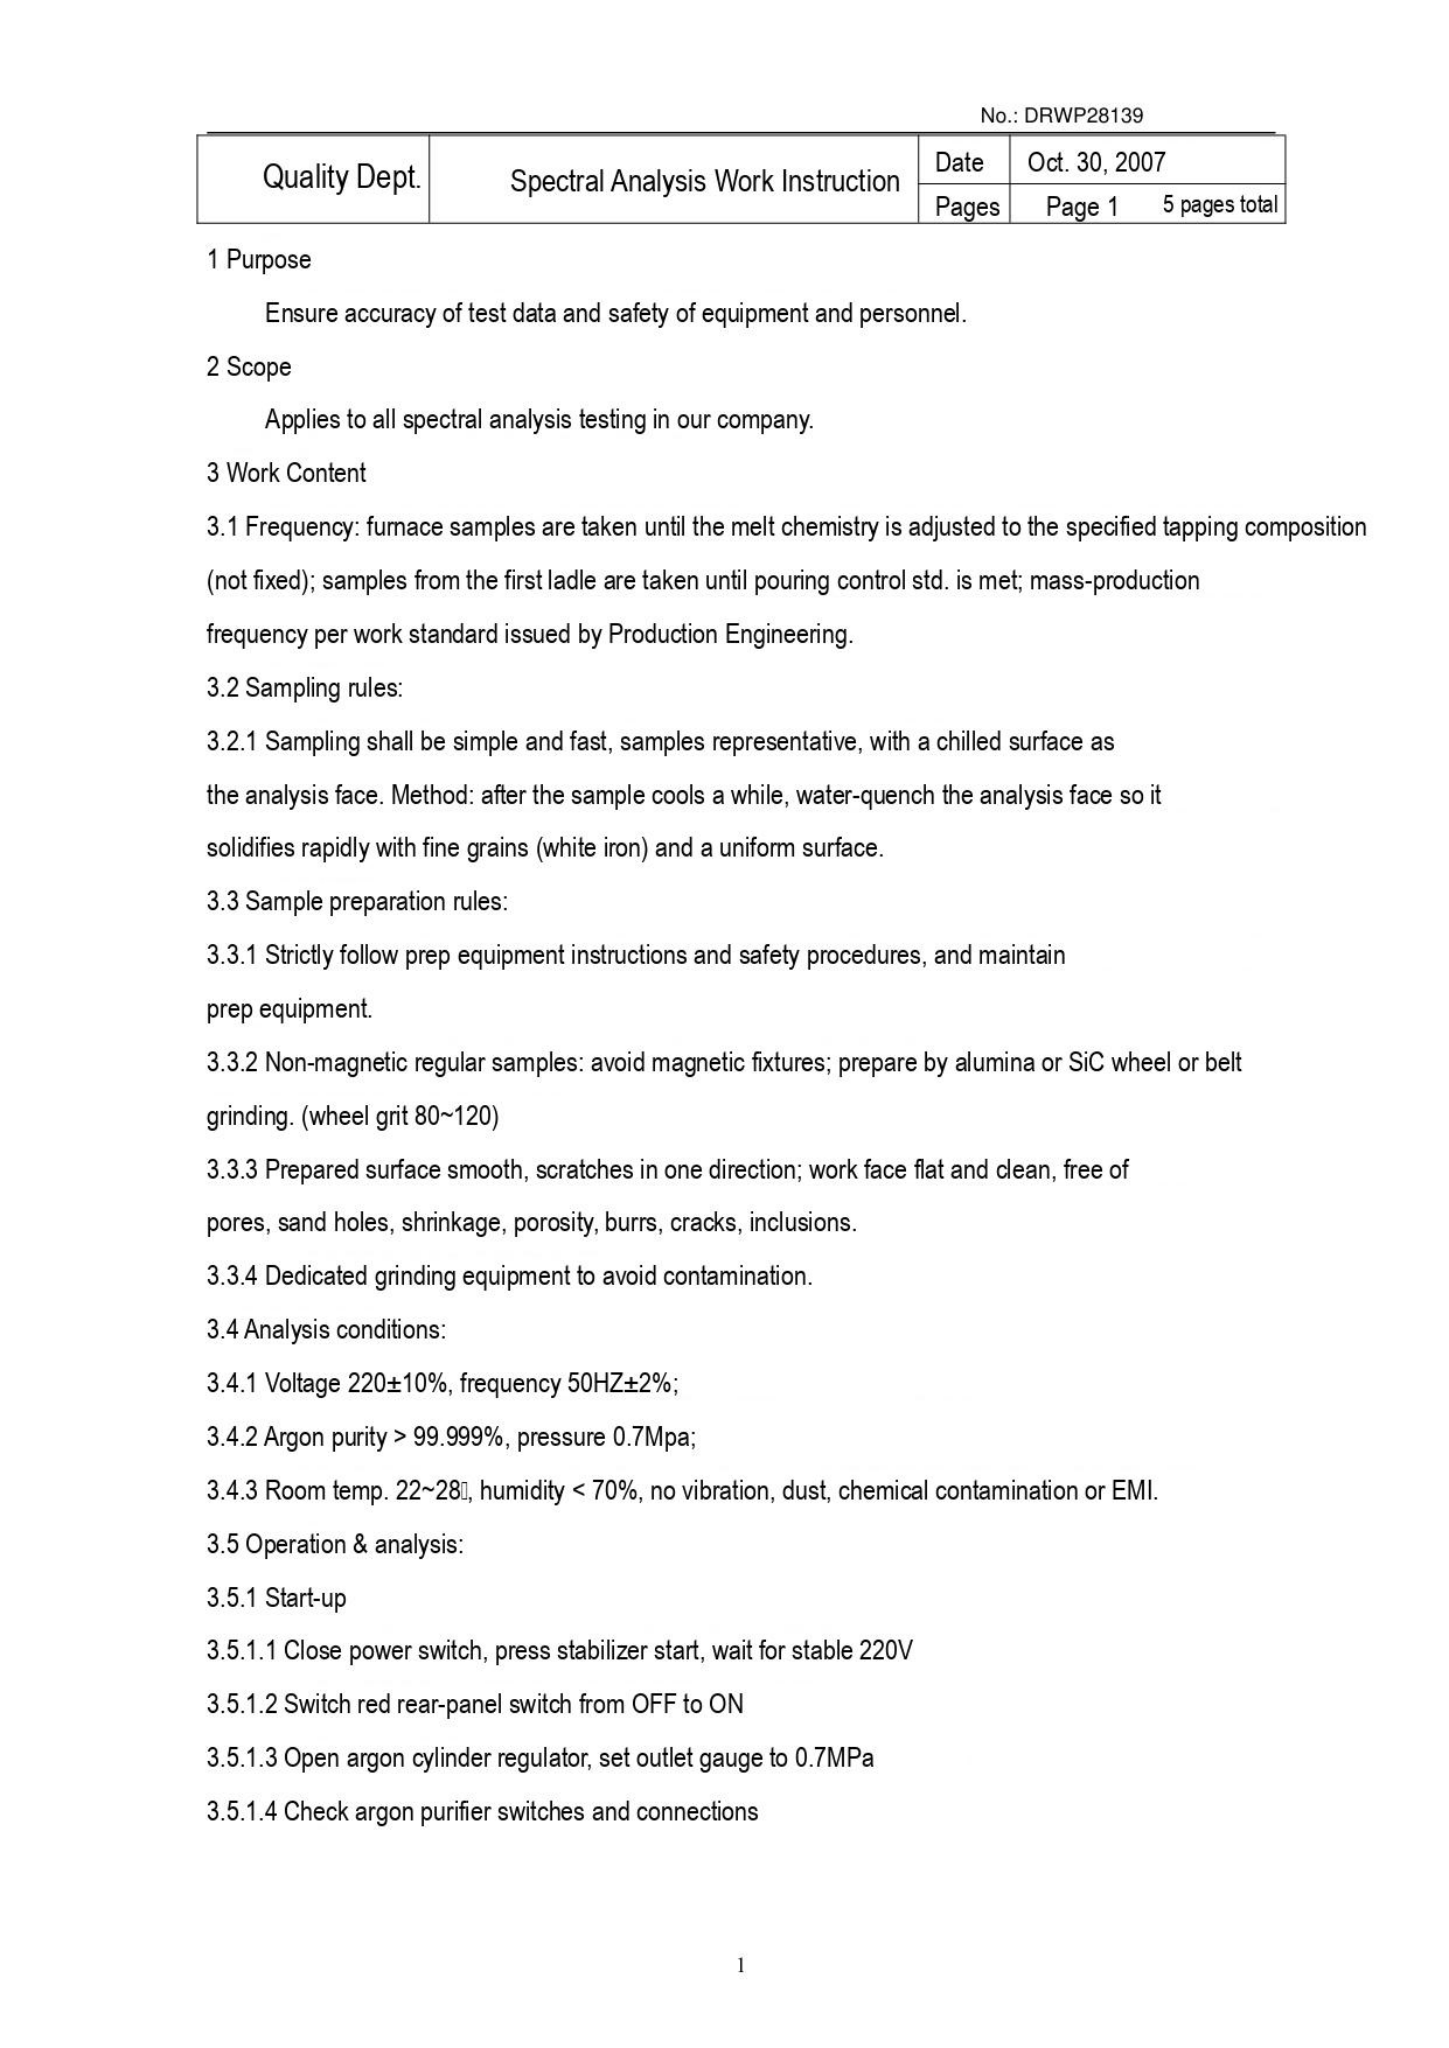No.: DRWP28139

| Quality Dept. | Spectral Analysis Work Instruction | Date | Oct. 30, 2007 | |
|---|---|---|---|---|
| | | Pages | Page 1 | 5 pages total |

1 Purpose

Ensure accuracy of test data and safety of equipment and personnel.

2 Scope

Applies to all spectral analysis testing in our company.

3 Work Content

3.1 Frequency: furnace samples are taken until the melt chemistry is adjusted to the specified tapping composition (not fixed); samples from the first ladle are taken until pouring control std. is met; mass-production frequency per work standard issued by Production Engineering.

3.2 Sampling rules:

3.2.1 Sampling shall be simple and fast, samples representative, with a chilled surface as the analysis face. Method: after the sample cools a while, water-quench the analysis face so it solidifies rapidly with fine grains (white iron) and a uniform surface.

3.3 Sample preparation rules:

3.3.1 Strictly follow prep equipment instructions and safety procedures, and maintain prep equipment.

3.3.2 Non-magnetic regular samples: avoid magnetic fixtures; prepare by alumina or SiC wheel or belt grinding. (wheel grit 80~120)

3.3.3 Prepared surface smooth, scratches in one direction; work face flat and clean, free of pores, sand holes, shrinkage, porosity, burrs, cracks, inclusions.

3.3.4 Dedicated grinding equipment to avoid contamination.

3.4 Analysis conditions:

3.4.1 Voltage 220±10%, frequency 50HZ±2%;

3.4.2 Argon purity > 99.999%, pressure 0.7Mpa;

3.4.3 Room temp. 22~28, humidity < 70%, no vibration, dust, chemical contamination or EMI.

3.5 Operation & analysis:

3.5.1 Start-up

3.5.1.1 Close power switch, press stabilizer start, wait for stable 220V

3.5.1.2 Switch red rear-panel switch from OFF to ON

3.5.1.3 Open argon cylinder regulator, set outlet gauge to 0.7MPa

3.5.1.4 Check argon purifier switches and connections

1
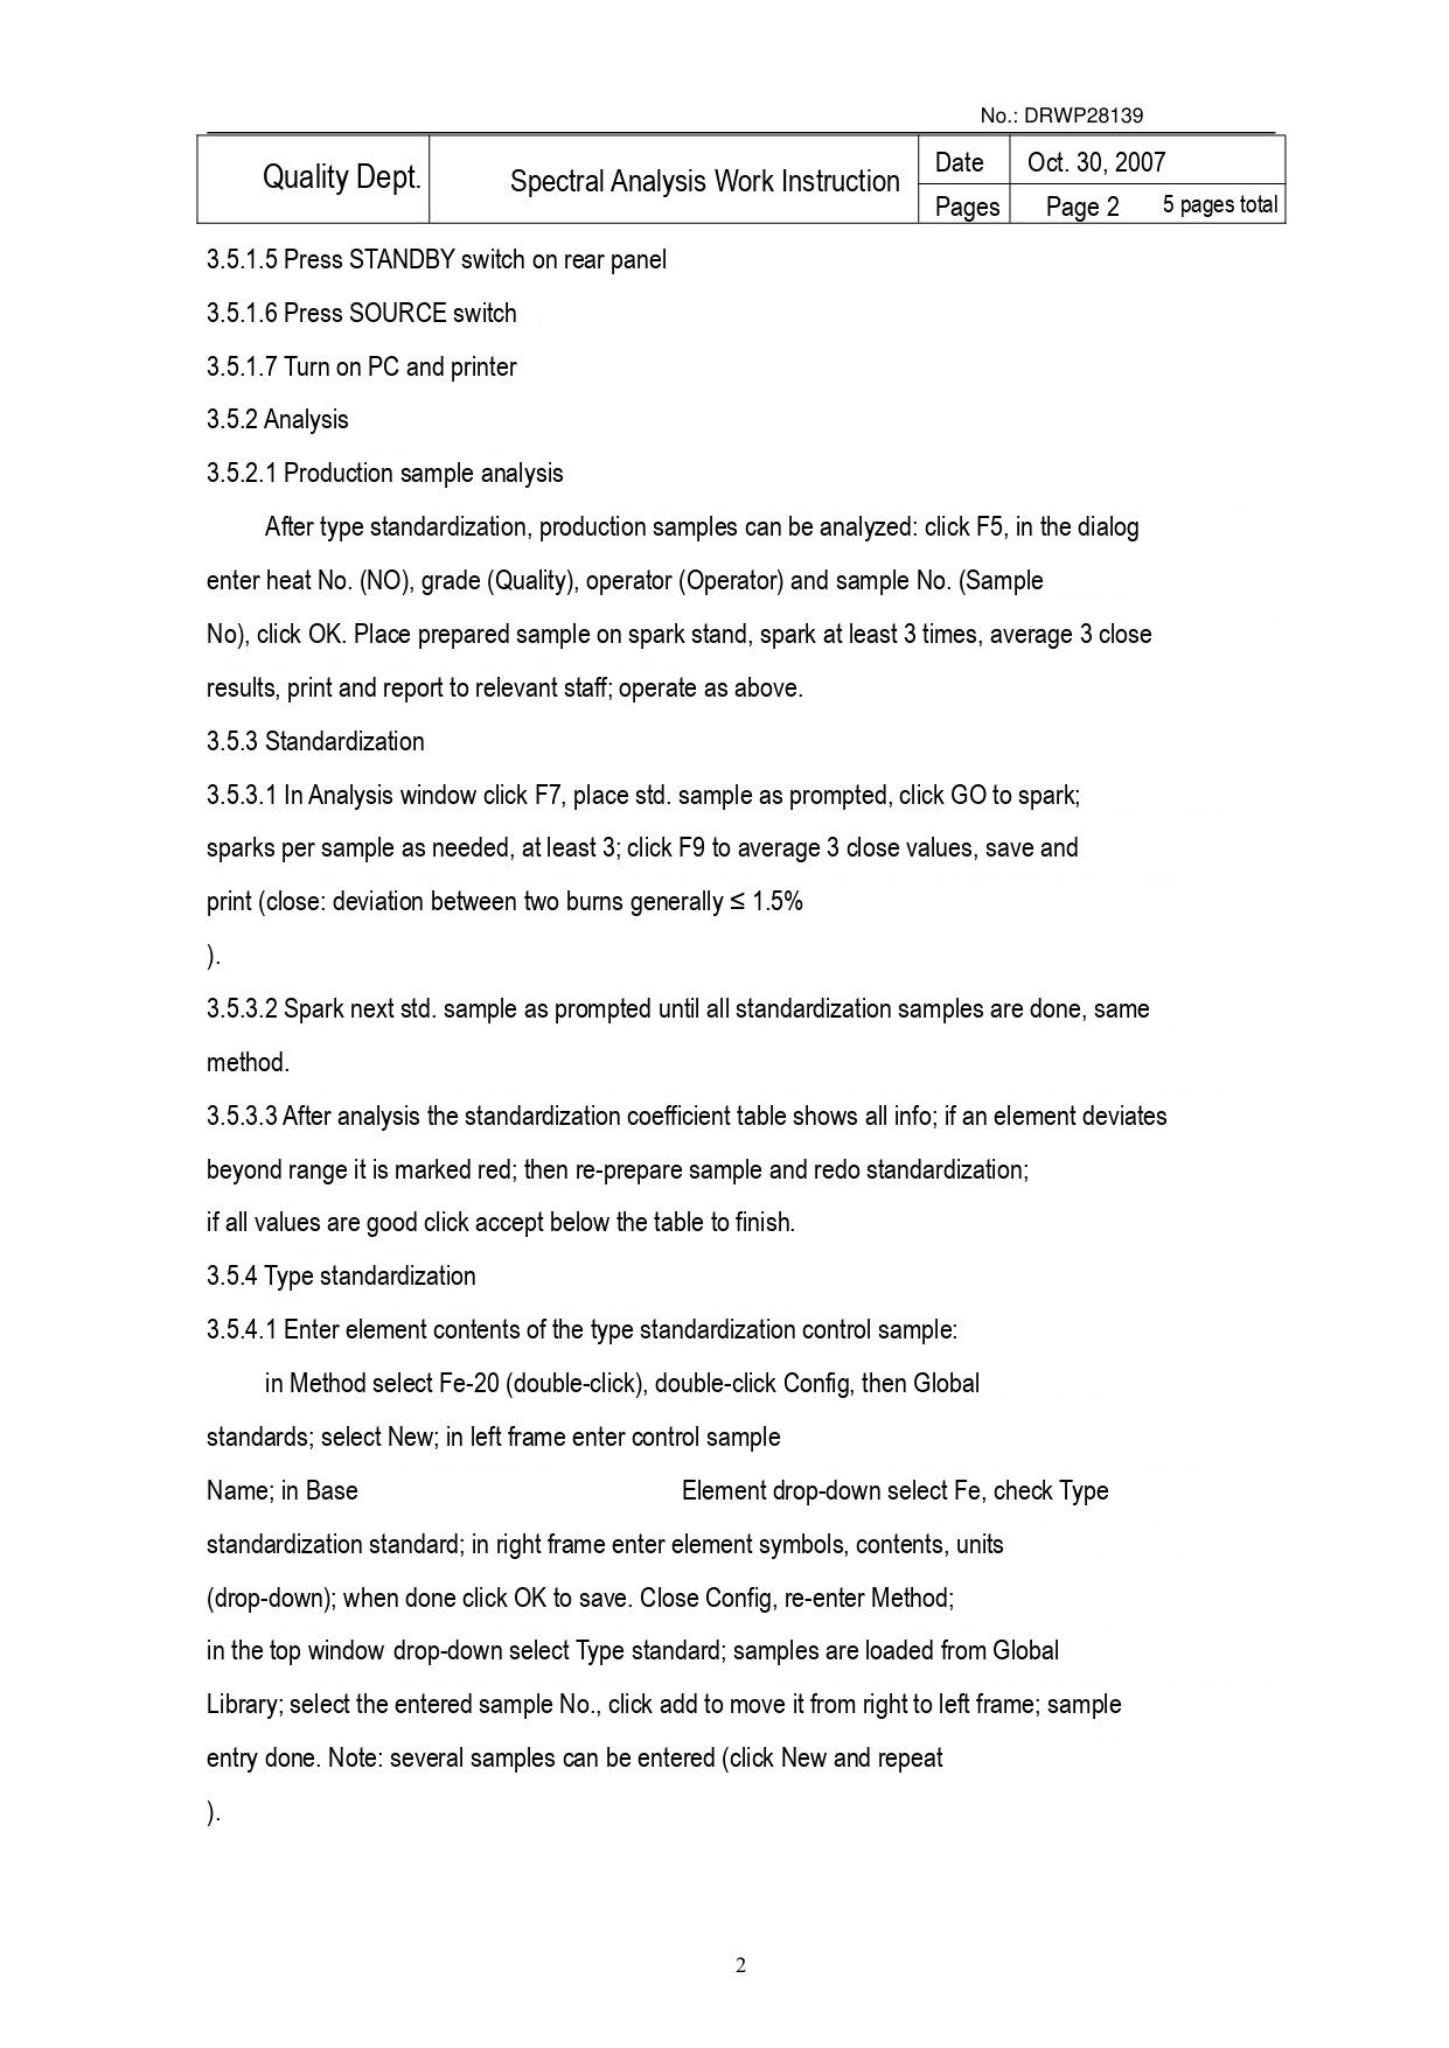No.: DRWP28139

| Quality Dept. | Spectral Analysis Work Instruction | Date | Oct. 30, 2007 | |
|---|---|---|---|---|
| | | Pages | Page 2 | 5 pages total |

3.5.1.5 Press STANDBY switch on rear panel

3.5.1.6 Press SOURCE switch

3.5.1.7 Turn on PC and printer

3.5.2 Analysis

3.5.2.1 Production sample analysis

After type standardization, production samples can be analyzed: click F5, in the dialog enter heat No. (NO), grade (Quality), operator (Operator) and sample No. (Sample No), click OK. Place prepared sample on spark stand, spark at least 3 times, average 3 close results, print and report to relevant staff; operate as above.

3.5.3 Standardization

3.5.3.1 In Analysis window click F7, place std. sample as prompted, click GO to spark; sparks per sample as needed, at least 3; click F9 to average 3 close values, save and print (close: deviation between two burns generally ≤ 1.5%
).

3.5.3.2 Spark next std. sample as prompted until all standardization samples are done, same method.

3.5.3.3 After analysis the standardization coefficient table shows all info; if an element deviates beyond range it is marked red; then re-prepare sample and redo standardization;
if all values are good click accept below the table to finish.

3.5.4 Type standardization

3.5.4.1 Enter element contents of the type standardization control sample:

in Method select Fe-20 (double-click), double-click Config, then Global standards; select New; in left frame enter control sample Name; in Base Element drop-down select Fe, check Type standardization standard; in right frame enter element symbols, contents, units (drop-down); when done click OK to save. Close Config, re-enter Method;
in the top window drop-down select Type standard; samples are loaded from Global Library; select the entered sample No., click add to move it from right to left frame; sample entry done. Note: several samples can be entered (click New and repeat
).

2
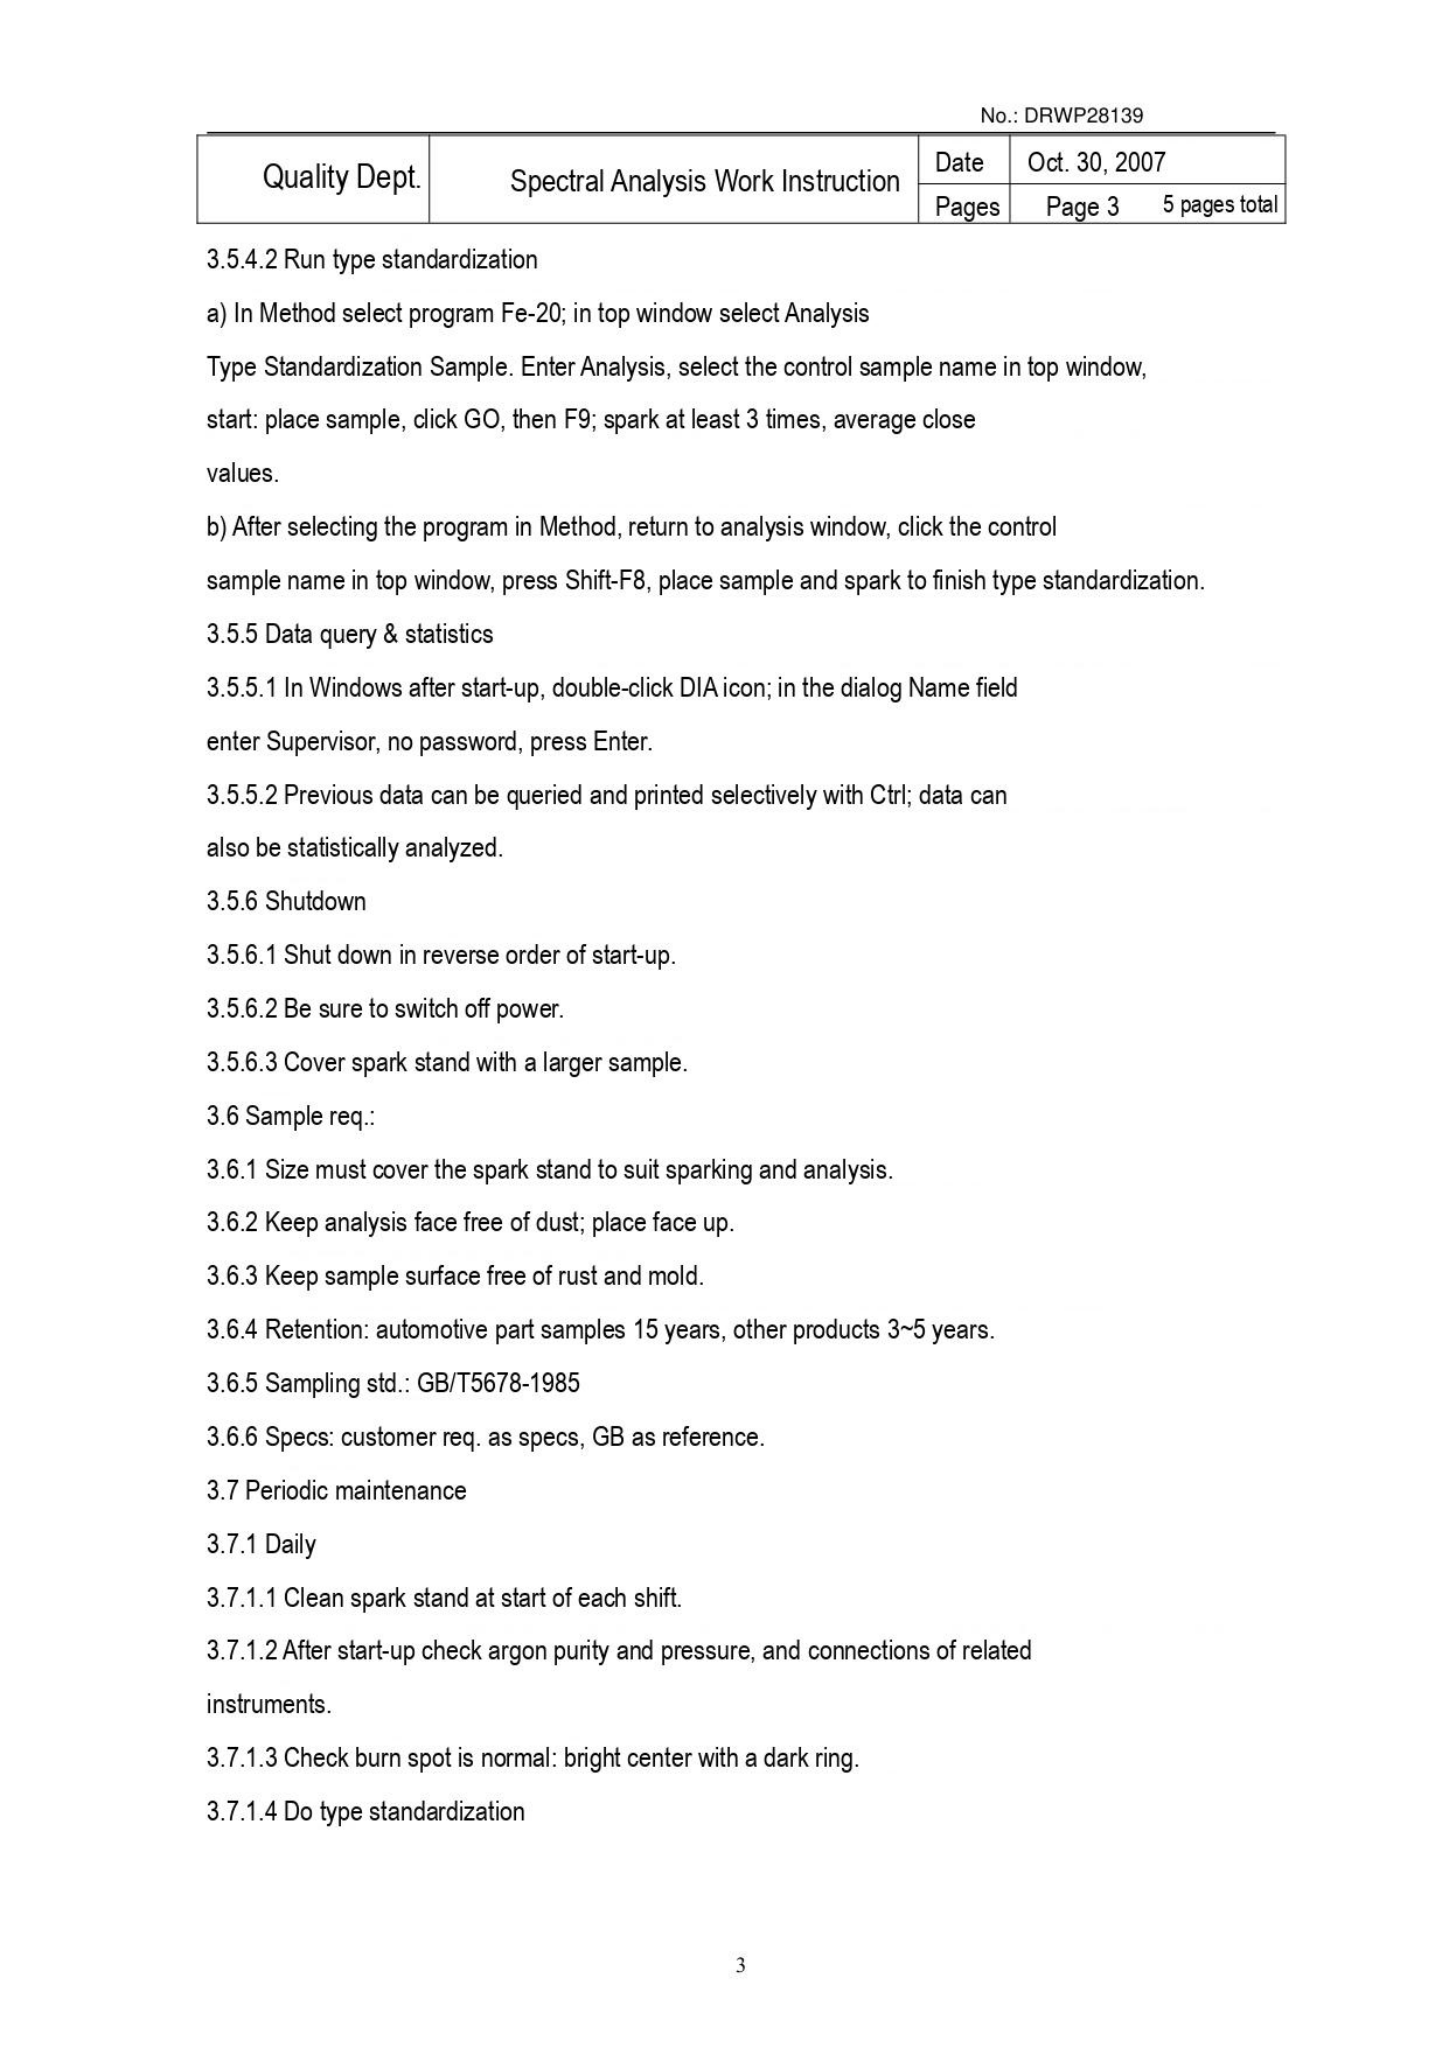No.: DRWP28139

| Quality Dept. | Spectral Analysis Work Instruction | Date | Oct. 30, 2007 | |
|---|---|---|---|---|
| | | Pages | Page 3 | 5 pages total |

3.5.4.2 Run type standardization

a) In Method select program Fe-20; in top window select Analysis

Type Standardization Sample. Enter Analysis, select the control sample name in top window,

start: place sample, click GO, then F9; spark at least 3 times, average close

values.

b) After selecting the program in Method, return to analysis window, click the control

sample name in top window, press Shift-F8, place sample and spark to finish type standardization.

3.5.5 Data query & statistics

3.5.5.1 In Windows after start-up, double-click DIA icon; in the dialog Name field

enter Supervisor, no password, press Enter.

3.5.5.2 Previous data can be queried and printed selectively with Ctrl; data can

also be statistically analyzed.

3.5.6 Shutdown

3.5.6.1 Shut down in reverse order of start-up.

3.5.6.2 Be sure to switch off power.

3.5.6.3 Cover spark stand with a larger sample.

3.6 Sample req.:

3.6.1 Size must cover the spark stand to suit sparking and analysis.

3.6.2 Keep analysis face free of dust; place face up.

3.6.3 Keep sample surface free of rust and mold.

3.6.4 Retention: automotive part samples 15 years, other products 3~5 years.

3.6.5 Sampling std.: GB/T5678-1985

3.6.6 Specs: customer req. as specs, GB as reference.

3.7 Periodic maintenance

3.7.1 Daily

3.7.1.1 Clean spark stand at start of each shift.

3.7.1.2 After start-up check argon purity and pressure, and connections of related

instruments.

3.7.1.3 Check burn spot is normal: bright center with a dark ring.

3.7.1.4 Do type standardization

3
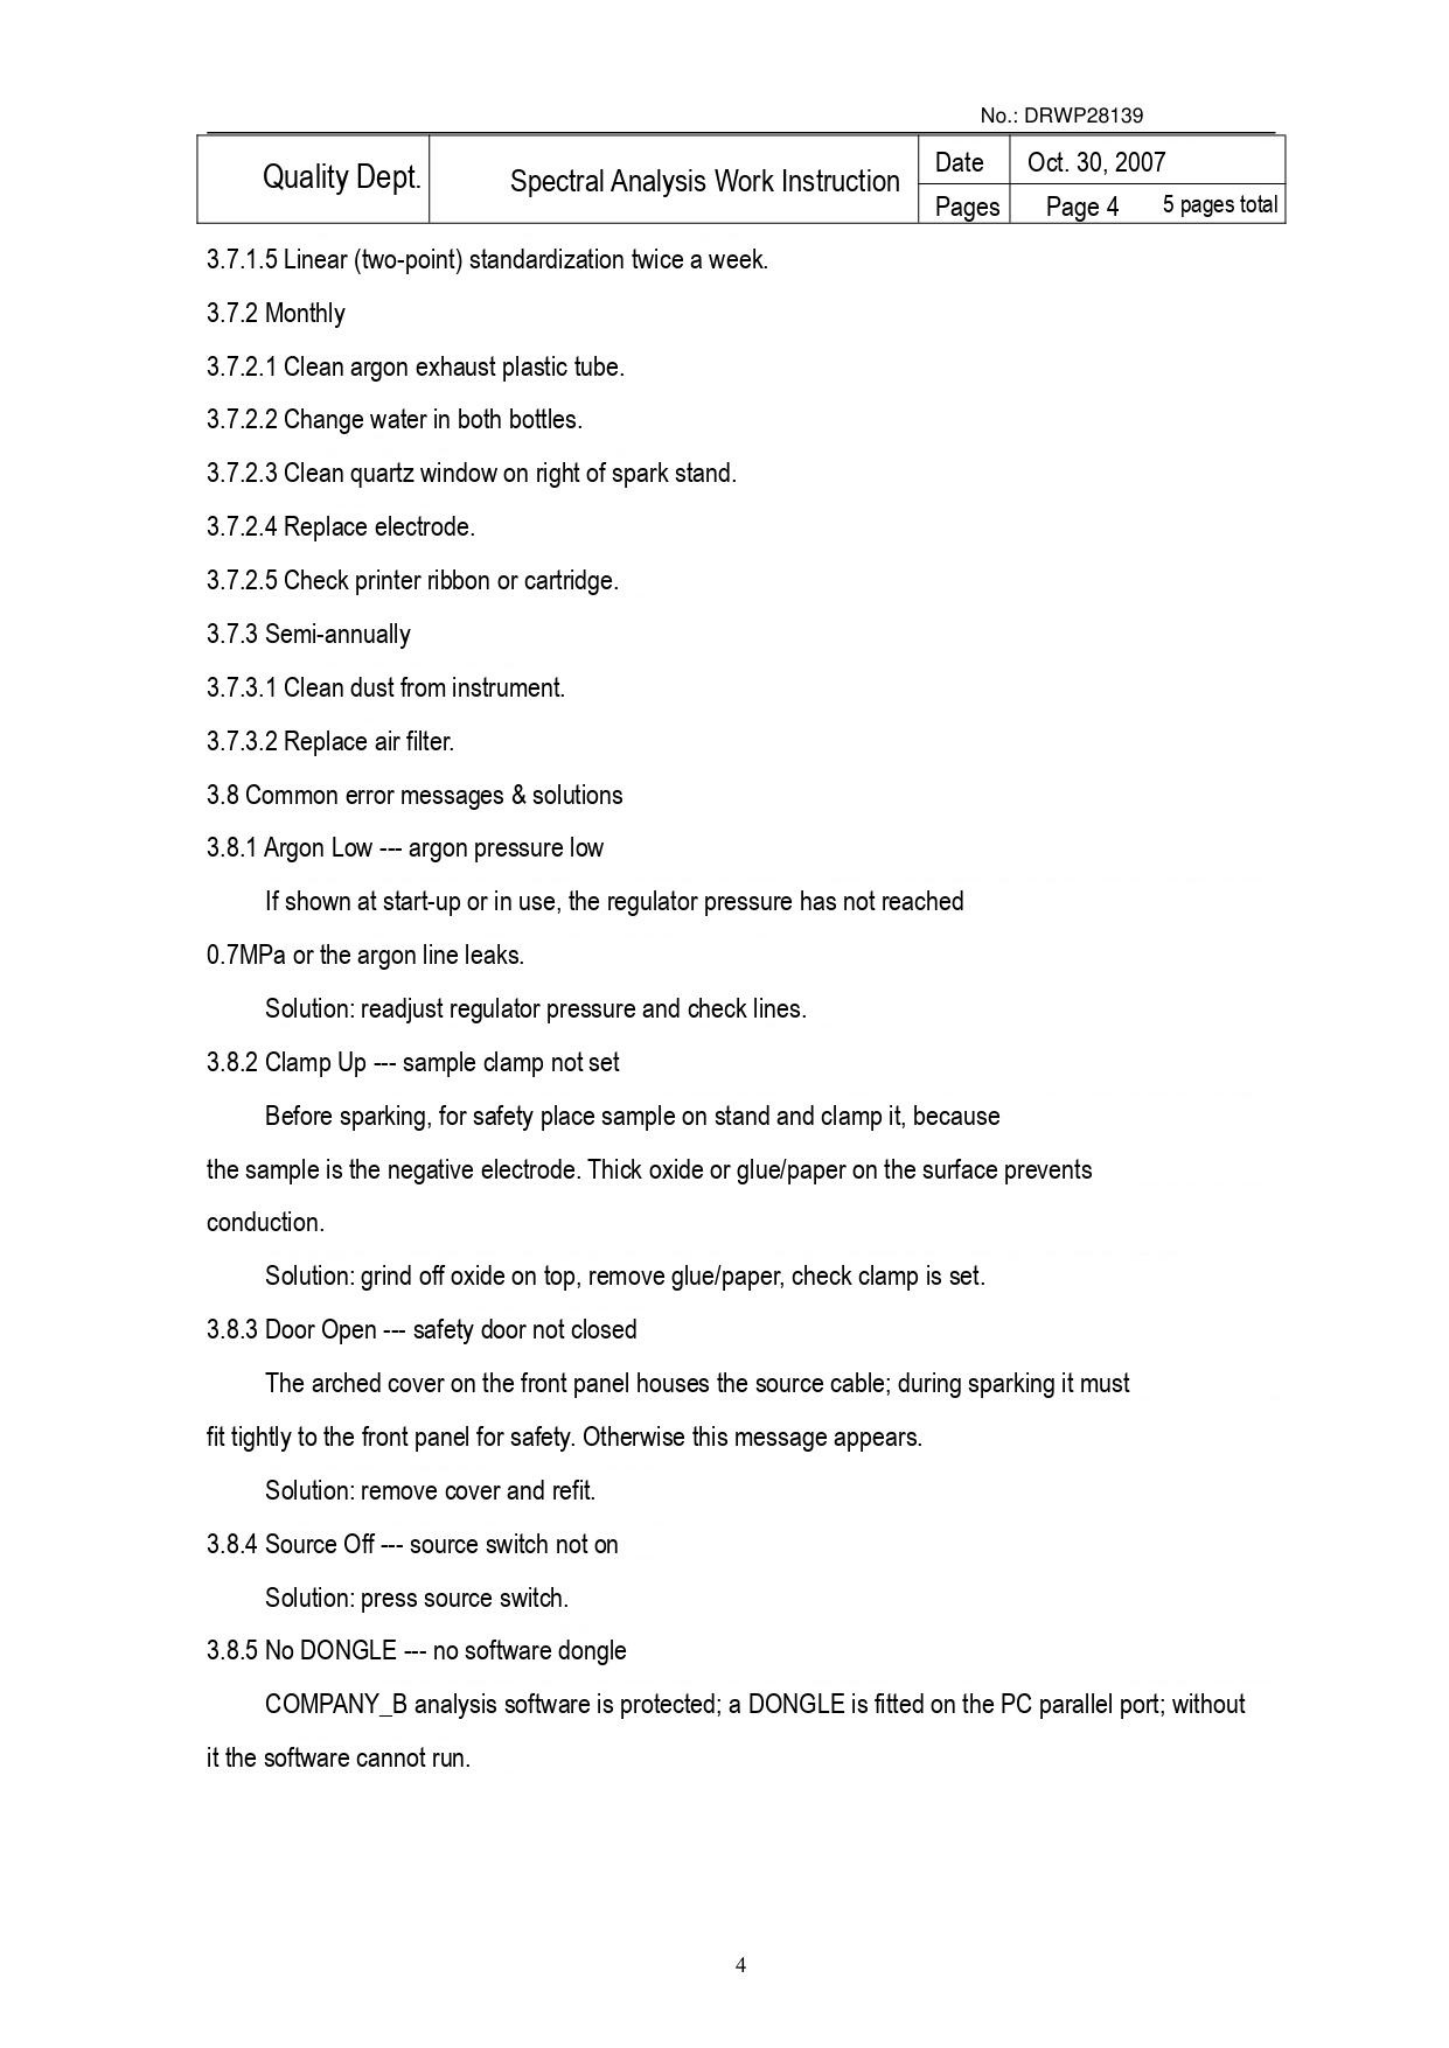No.: DRWP28139

| Quality Dept. | Spectral Analysis Work Instruction | Date | Oct. 30, 2007 | |
|---|---|---|---|---|
| | | Pages | Page 4 | 5 pages total |

3.7.1.5 Linear (two-point) standardization twice a week.

3.7.2 Monthly

3.7.2.1 Clean argon exhaust plastic tube.

3.7.2.2 Change water in both bottles.

3.7.2.3 Clean quartz window on right of spark stand.

3.7.2.4 Replace electrode.

3.7.2.5 Check printer ribbon or cartridge.

3.7.3 Semi-annually

3.7.3.1 Clean dust from instrument.

3.7.3.2 Replace air filter.

3.8 Common error messages & solutions

3.8.1 Argon Low --- argon pressure low

If shown at start-up or in use, the regulator pressure has not reached 0.7MPa or the argon line leaks.

Solution: readjust regulator pressure and check lines.

3.8.2 Clamp Up --- sample clamp not set

Before sparking, for safety place sample on stand and clamp it, because the sample is the negative electrode. Thick oxide or glue/paper on the surface prevents conduction.

Solution: grind off oxide on top, remove glue/paper, check clamp is set.

3.8.3 Door Open --- safety door not closed

The arched cover on the front panel houses the source cable; during sparking it must fit tightly to the front panel for safety. Otherwise this message appears.

Solution: remove cover and refit.

3.8.4 Source Off --- source switch not on

Solution: press source switch.

3.8.5 No DONGLE --- no software dongle

COMPANY_B analysis software is protected; a DONGLE is fitted on the PC parallel port; without it the software cannot run.

4
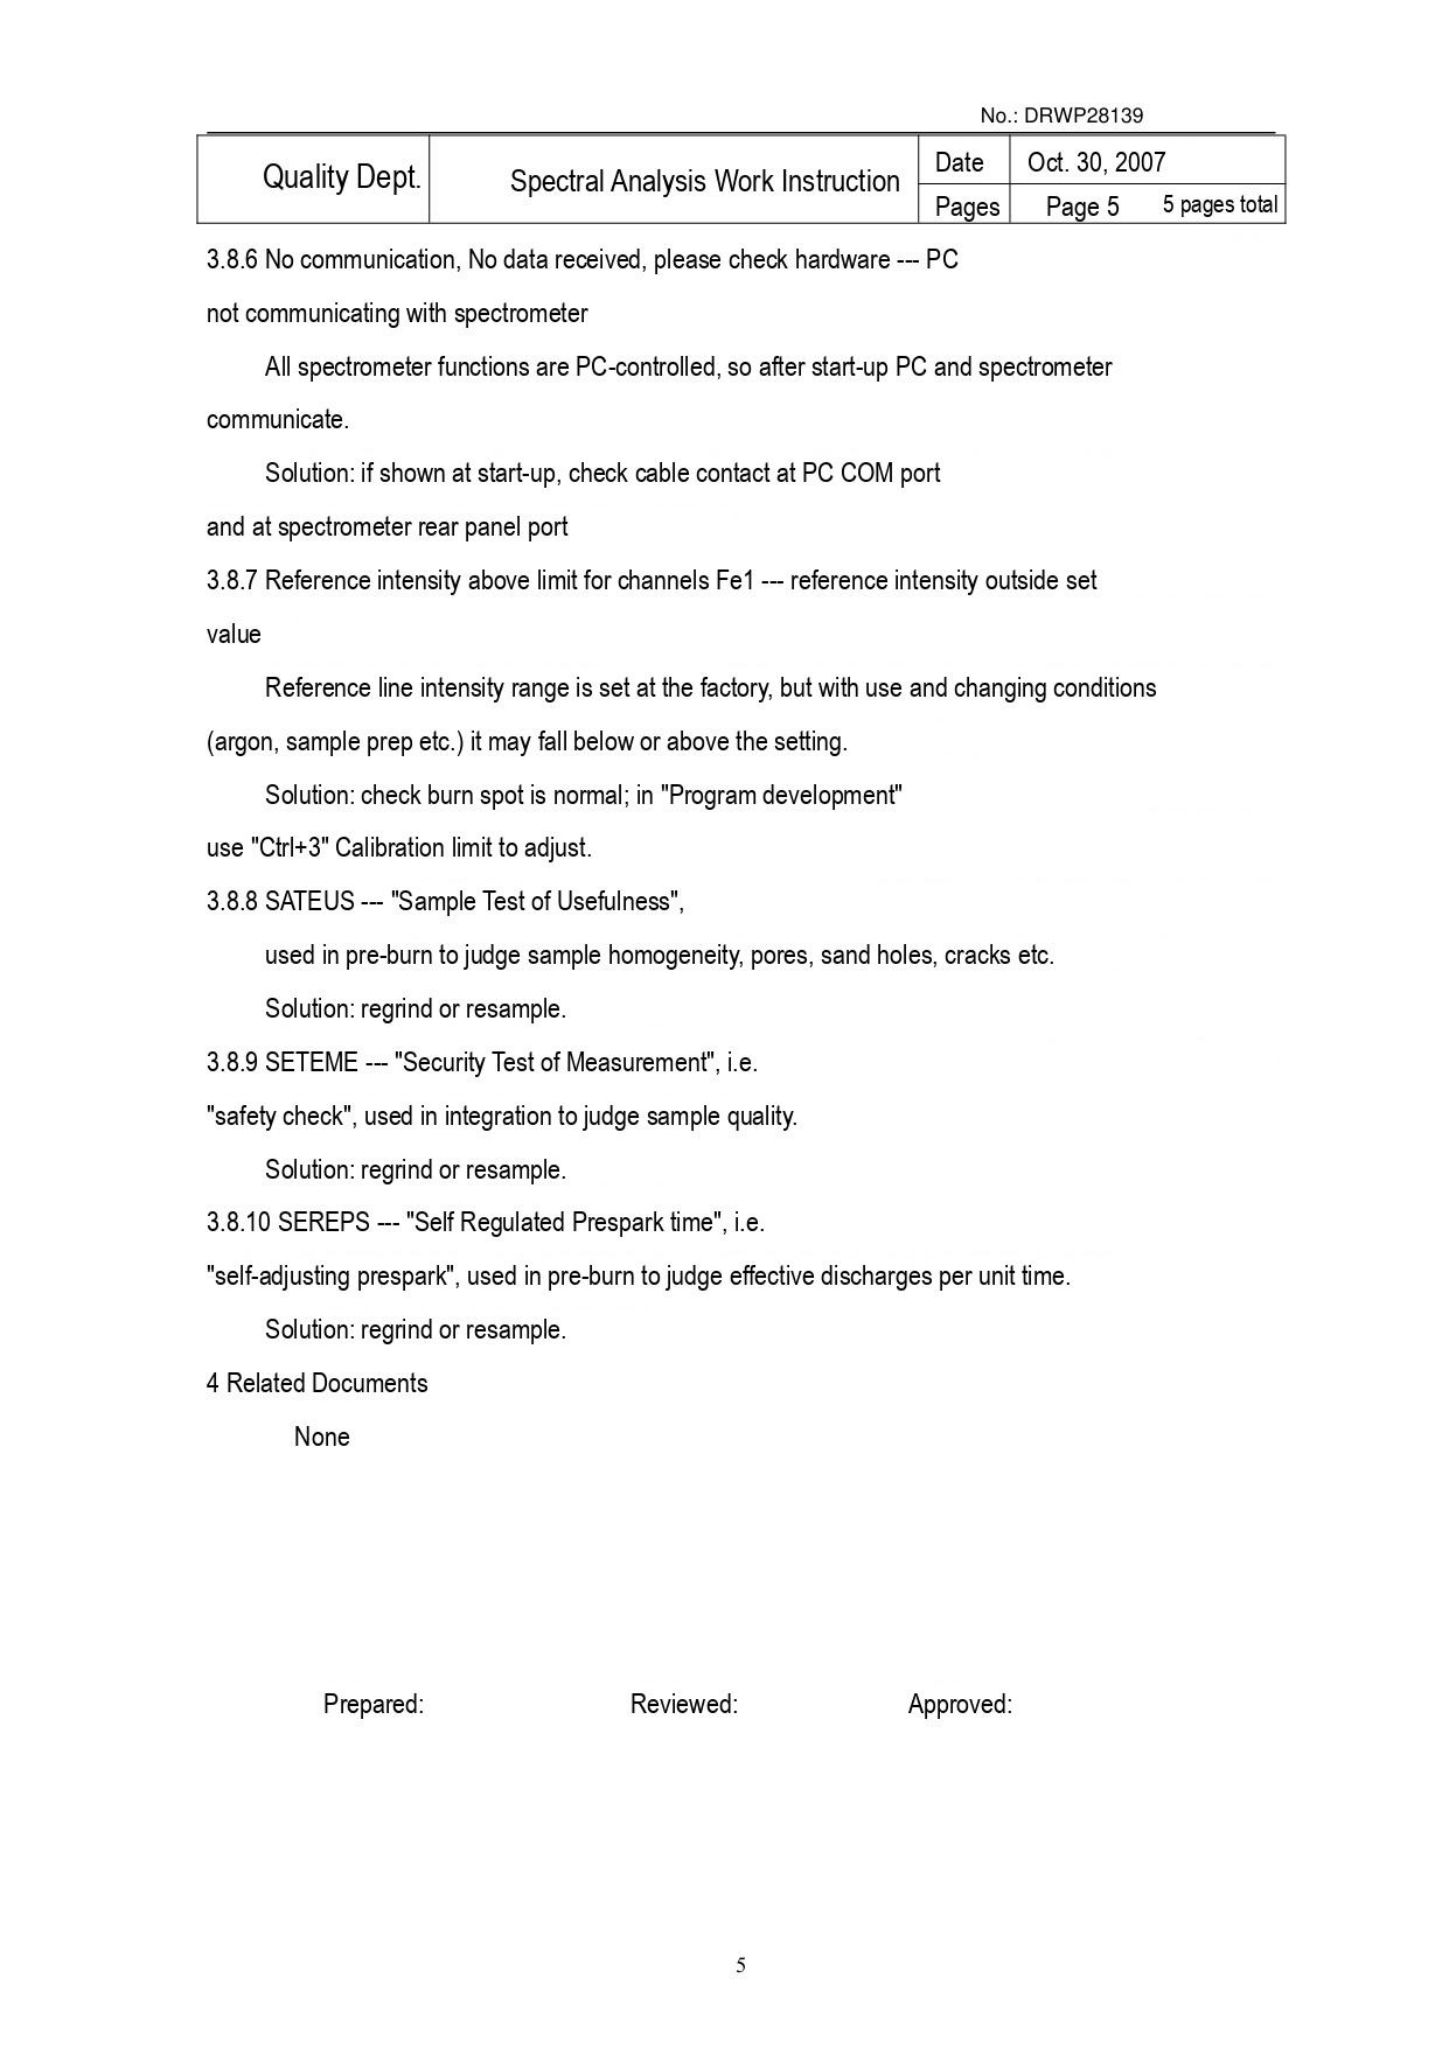No.: DRWP28139

| Quality Dept. | Spectral Analysis Work Instruction | Date | Oct. 30, 2007 | |
|---|---|---|---|---|
| | | Pages | Page 5 | 5 pages total |

3.8.6 No communication, No data received, please check hardware --- PC not communicating with spectrometer

All spectrometer functions are PC-controlled, so after start-up PC and spectrometer communicate.

Solution: if shown at start-up, check cable contact at PC COM port and at spectrometer rear panel port

3.8.7 Reference intensity above limit for channels Fe1 --- reference intensity outside set value

Reference line intensity range is set at the factory, but with use and changing conditions (argon, sample prep etc.) it may fall below or above the setting.

Solution: check burn spot is normal; in "Program development" use "Ctrl+3" Calibration limit to adjust.

3.8.8 SATEUS --- "Sample Test of Usefulness",

used in pre-burn to judge sample homogeneity, pores, sand holes, cracks etc.

Solution: regrind or resample.

3.8.9 SETEME --- "Security Test of Measurement", i.e. "safety check", used in integration to judge sample quality.

Solution: regrind or resample.

3.8.10 SEREPS --- "Self Regulated Prespark time", i.e. "self-adjusting prespark", used in pre-burn to judge effective discharges per unit time.

Solution: regrind or resample.

4 Related Documents

None

Prepared: Reviewed: Approved:

5